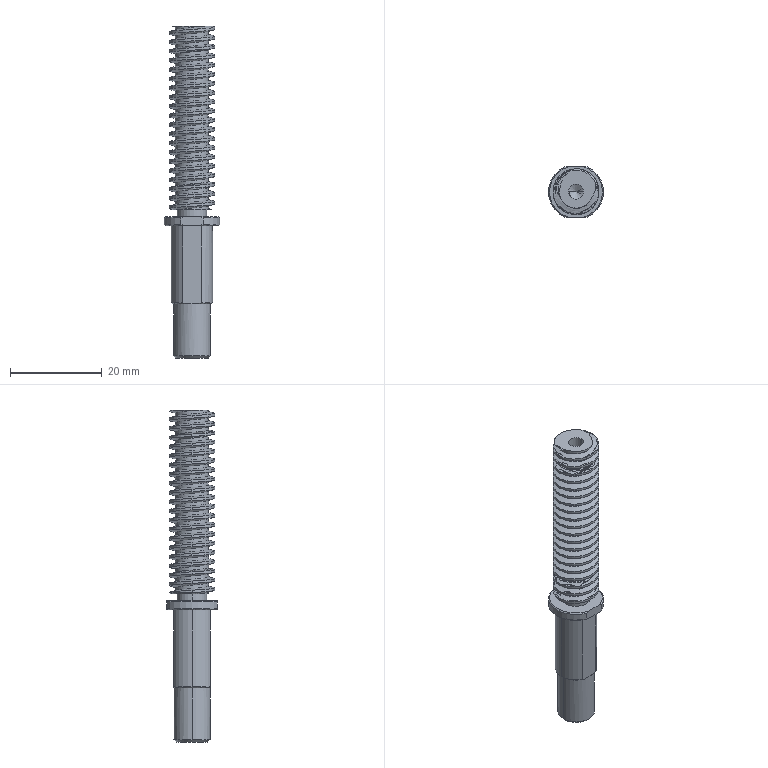Part | NX | features BREP 1 | 1 solid | 87 faces | box 12 x 11 x 72.3 mm | volume 3949 mm3 | cylinder 56 | cone 17 | plane 12 | spline 2 | commonest cylinder face diameters 10 x41 3.3 x4 9 x3 12 x3 6.5 x2 8 x2